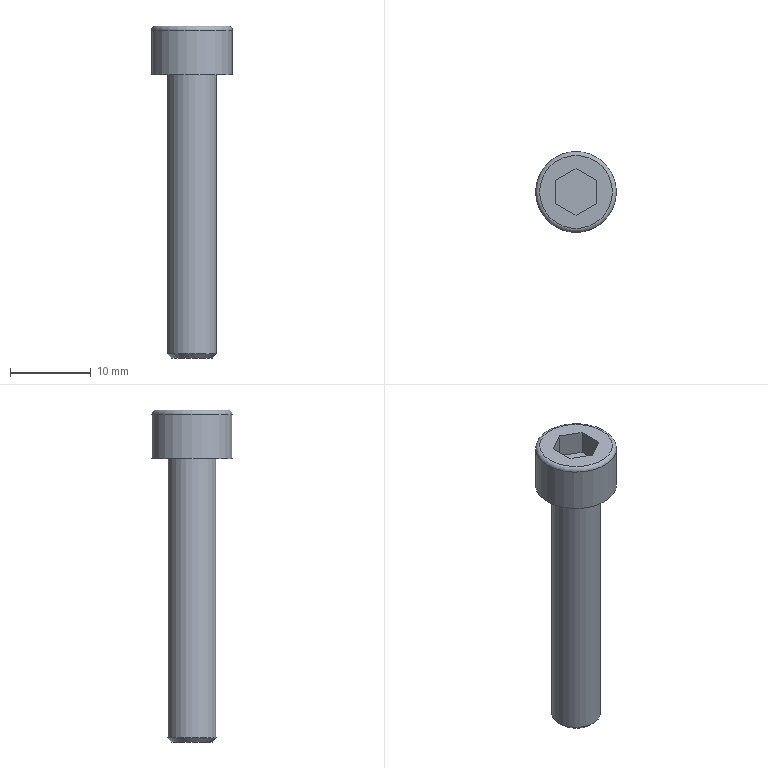Part | STEP file | lll_id66_x_t | 1 solid | 14 faces | box 10 x 10 x 41 mm | volume 1392 mm3 | plane 10 | cylinder 2 | torus 1 | cone 1 | commonest cylinder face diameters 6 x1 10 x1
STEP:
#1=CARTESIAN_POINT('',(24.,58.443,-12.5));
#2=VERTEX_POINT('',#1);
#3=CARTESIAN_POINT('',(21.5,59.887,-12.5));
#4=VERTEX_POINT('',#3);
#5=CARTESIAN_POINT('',(24.,58.443,-12.5));
#6=DIRECTION('',(-0.866,0.5,0.));
#7=VECTOR('',#6,1.);
#8=LINE('',#5,#7);
#9=EDGE_CURVE('',#2,#4,#8,.T.);
#10=ORIENTED_EDGE('',*,*,#9,.F.);
#11=CARTESIAN_POINT('',(24.,55.557,-12.5));
#12=VERTEX_POINT('',#11);
#13=CARTESIAN_POINT('',(24.,55.557,-12.5));
#14=DIRECTION('',(0.,1.,0.));
#15=VECTOR('',#14,1.);
#16=LINE('',#13,#15);
#17=EDGE_CURVE('',#12,#2,#16,.T.);
#18=ORIENTED_EDGE('',*,*,#17,.F.);
#19=CARTESIAN_POINT('',(21.5,54.113,-12.5));
#20=VERTEX_POINT('',#19);
#21=CARTESIAN_POINT('',(21.5,54.113,-12.5));
#22=DIRECTION('',(0.866,0.5,0.));
#23=VECTOR('',#22,1.);
#24=LINE('',#21,#23);
#25=EDGE_CURVE('',#20,#12,#24,.T.);
#26=ORIENTED_EDGE('',*,*,#25,.F.);
#27=CARTESIAN_POINT('',(19.,55.557,-12.5));
#28=VERTEX_POINT('',#27);
#29=CARTESIAN_POINT('',(19.,55.557,-12.5));
#30=DIRECTION('',(0.866,-0.5,0.));
#31=VECTOR('',#30,1.);
#32=LINE('',#29,#31);
#33=EDGE_CURVE('',#28,#20,#32,.T.);
#34=ORIENTED_EDGE('',*,*,#33,.F.);
#35=CARTESIAN_POINT('',(19.,58.443,-12.5));
#36=VERTEX_POINT('',#35);
#37=CARTESIAN_POINT('',(19.,58.443,-12.5));
#38=DIRECTION('',(0.,-1.,0.));
#39=VECTOR('',#38,1.);
#40=LINE('',#37,#39);
#41=EDGE_CURVE('',#36,#28,#40,.T.);
#42=ORIENTED_EDGE('',*,*,#41,.F.);
#43=CARTESIAN_POINT('',(21.5,59.887,-12.5));
#44=DIRECTION('',(-0.866,-0.5,0.));
#45=VECTOR('',#44,1.);
#46=LINE('',#43,#45);
#47=EDGE_CURVE('',#4,#36,#46,.T.);
#48=ORIENTED_EDGE('',*,*,#47,.F.);
#49=EDGE_LOOP('',(#10,#18,#26,#34,#42,#48));
#50=FACE_BOUND('',#49,.T.);
#51=CARTESIAN_POINT('',(26.,57.,-12.5));
#52=VERTEX_POINT('',#51);
#53=CARTESIAN_POINT('',(21.5,57.,-12.5));
#54=DIRECTION('',(0.,0.,1.));
#55=DIRECTION('',(1.,0.,0.));
#56=AXIS2_PLACEMENT_3D('',#53,#54,#55);
#57=CIRCLE('',#56,4.5);
#58=EDGE_CURVE('',#52,#52,#57,.T.);
#59=ORIENTED_EDGE('',*,*,#58,.T.);
#60=EDGE_LOOP('',(#59));
#61=FACE_BOUND('',#60,.T.);
#62=CARTESIAN_POINT('',(21.5,57.,-12.5));
#63=DIRECTION('',(0.,0.,1.));
#64=DIRECTION('',(1.,0.,0.));
#65=AXIS2_PLACEMENT_3D('',#62,#63,#64);
#66=PLANE('',#65);
#67=ADVANCED_FACE('',(#50,#61),#66,.T.);
#68=CARTESIAN_POINT('',(18.5,57.,-18.5));
#69=VERTEX_POINT('',#68);
#70=CARTESIAN_POINT('',(21.5,57.,-18.5));
#71=DIRECTION('',(0.,0.,-1.));
#72=DIRECTION('',(-1.,0.,0.));
#73=AXIS2_PLACEMENT_3D('',#70,#71,#72);
#74=CIRCLE('',#73,3.);
#75=EDGE_CURVE('',#69,#69,#74,.T.);
#76=ORIENTED_EDGE('',*,*,#75,.F.);
#77=EDGE_LOOP('',(#76));
#78=FACE_BOUND('',#77,.T.);
#79=CARTESIAN_POINT('',(26.5,57.,-18.5));
#80=VERTEX_POINT('',#79);
#81=CARTESIAN_POINT('',(21.5,57.,-18.5));
#82=DIRECTION('',(0.,0.,1.));
#83=DIRECTION('',(1.,0.,0.));
#84=AXIS2_PLACEMENT_3D('',#81,#82,#83);
#85=CIRCLE('',#84,5.);
#86=EDGE_CURVE('',#80,#80,#85,.T.);
#87=ORIENTED_EDGE('',*,*,#86,.F.);
#88=EDGE_LOOP('',(#87));
#89=FACE_BOUND('',#88,.T.);
#90=CARTESIAN_POINT('',(21.5,57.,-18.5));
#91=DIRECTION('',(0.,0.,-1.));
#92=DIRECTION('',(-1.,0.,0.));
#93=AXIS2_PLACEMENT_3D('',#90,#91,#92);
#94=PLANE('',#93);
#95=ADVANCED_FACE('',(#78,#89),#94,.T.);
#96=CARTESIAN_POINT('',(26.5,57.,-13.));
#97=VERTEX_POINT('',#96);
#98=CARTESIAN_POINT('',(21.5,57.,-13.));
#99=DIRECTION('',(0.,0.,-1.));
#100=DIRECTION('',(1.,0.,0.));
#101=AXIS2_PLACEMENT_3D('',#98,#99,#100);
#102=CIRCLE('',#101,5.);
#103=EDGE_CURVE('',#97,#97,#102,.T.);
#104=ORIENTED_EDGE('',*,*,#103,.T.);
#105=EDGE_LOOP('',(#104));
#106=FACE_BOUND('',#105,.T.);
#107=ORIENTED_EDGE('',*,*,#86,.T.);
#108=EDGE_LOOP('',(#107));
#109=FACE_BOUND('',#108,.T.);
#110=CARTESIAN_POINT('',(21.5,57.,-18.5));
#111=DIRECTION('',(0.,0.,1.));
#112=DIRECTION('',(1.,0.,0.));
#113=AXIS2_PLACEMENT_3D('',#110,#111,#112);
#114=CYLINDRICAL_SURFACE('',#113,5.);
#115=ADVANCED_FACE('',(#106,#109),#114,.T.);
#116=ORIENTED_EDGE('',*,*,#58,.F.);
#117=EDGE_LOOP('',(#116));
#118=FACE_BOUND('',#117,.T.);
#119=ORIENTED_EDGE('',*,*,#103,.F.);
#120=EDGE_LOOP('',(#119));
#121=FACE_BOUND('',#120,.T.);
#122=CARTESIAN_POINT('',(21.5,57.,-13.));
#123=DIRECTION('',(0.,0.,1.));
#124=DIRECTION('',(1.,0.,0.));
#125=AXIS2_PLACEMENT_3D('',#122,#123,#124);
#126=TOROIDAL_SURFACE('',#125,4.5,0.5);
#127=ADVANCED_FACE('',(#118,#121),#126,.T.);
#128=CARTESIAN_POINT('',(19.,57.,-53.5));
#129=VERTEX_POINT('',#128);
#130=CARTESIAN_POINT('',(21.5,57.,-53.5));
#131=DIRECTION('',(0.,0.,-1.));
#132=DIRECTION('',(-1.,0.,0.));
#133=AXIS2_PLACEMENT_3D('',#130,#131,#132);
#134=CIRCLE('',#133,2.5);
#135=EDGE_CURVE('',#129,#129,#134,.T.);
#136=ORIENTED_EDGE('',*,*,#135,.T.);
#137=EDGE_LOOP('',(#136));
#138=FACE_OUTER_BOUND('',#137,.T.);
#139=CARTESIAN_POINT('',(21.5,57.,-53.5));
#140=DIRECTION('',(0.,0.,-1.));
#141=DIRECTION('',(-1.,0.,0.));
#142=AXIS2_PLACEMENT_3D('',#139,#140,#141);
#143=PLANE('',#142);
#144=ADVANCED_FACE('',(#138),#143,.T.);
#145=ORIENTED_EDGE('',*,*,#75,.T.);
#146=EDGE_LOOP('',(#145));
#147=FACE_BOUND('',#146,.T.);
#148=CARTESIAN_POINT('',(18.5,57.,-53.));
#149=VERTEX_POINT('',#148);
#150=CARTESIAN_POINT('',(21.5,57.,-53.));
#151=DIRECTION('',(0.,0.,1.));
#152=DIRECTION('',(-1.,0.,0.));
#153=AXIS2_PLACEMENT_3D('',#150,#151,#152);
#154=CIRCLE('',#153,3.);
#155=EDGE_CURVE('',#149,#149,#154,.T.);
#156=ORIENTED_EDGE('',*,*,#155,.T.);
#157=EDGE_LOOP('',(#156));
#158=FACE_BOUND('',#157,.T.);
#159=CARTESIAN_POINT('',(21.5,57.,-53.5));
#160=DIRECTION('',(0.,0.,1.));
#161=DIRECTION('',(1.,0.,0.));
#162=AXIS2_PLACEMENT_3D('',#159,#160,#161);
#163=CYLINDRICAL_SURFACE('',#162,3.);
#164=ADVANCED_FACE('',(#147,#158),#163,.T.);
#165=ORIENTED_EDGE('',*,*,#135,.F.);
#166=EDGE_LOOP('',(#165));
#167=FACE_BOUND('',#166,.T.);
#168=ORIENTED_EDGE('',*,*,#155,.F.);
#169=EDGE_LOOP('',(#168));
#170=FACE_BOUND('',#169,.T.);
#171=CARTESIAN_POINT('',(21.5,57.,-53.));
#172=DIRECTION('',(0.,0.,1.));
#173=DIRECTION('',(1.,0.,0.));
#174=AXIS2_PLACEMENT_3D('',#171,#172,#173);
#175=CONICAL_SURFACE('',#174,3.,45.);
#176=ADVANCED_FACE('',(#167,#170),#175,.T.);
#177=CARTESIAN_POINT('',(24.,58.443,-15.5));
#178=VERTEX_POINT('',#177);
#179=CARTESIAN_POINT('',(21.5,59.887,-15.5));
#180=VERTEX_POINT('',#179);
#181=CARTESIAN_POINT('',(24.,58.443,-15.5));
#182=DIRECTION('',(-0.866,0.5,0.));
#183=VECTOR('',#182,1.);
#184=LINE('',#181,#183);
#185=EDGE_CURVE('',#178,#180,#184,.T.);
#186=ORIENTED_EDGE('',*,*,#185,.F.);
#187=CARTESIAN_POINT('',(24.,58.443,-12.5));
#188=DIRECTION('',(0.,0.,-1.));
#189=VECTOR('',#188,1.);
#190=LINE('',#187,#189);
#191=EDGE_CURVE('',#2,#178,#190,.T.);
#192=ORIENTED_EDGE('',*,*,#191,.F.);
#193=ORIENTED_EDGE('',*,*,#9,.T.);
#194=CARTESIAN_POINT('',(21.5,59.887,-12.5));
#195=DIRECTION('',(0.,0.,-1.));
#196=VECTOR('',#195,1.);
#197=LINE('',#194,#196);
#198=EDGE_CURVE('',#4,#180,#197,.T.);
#199=ORIENTED_EDGE('',*,*,#198,.T.);
#200=EDGE_LOOP('',(#186,#192,#193,#199));
#201=FACE_OUTER_BOUND('',#200,.T.);
#202=CARTESIAN_POINT('',(24.,58.443,-12.5));
#203=DIRECTION('',(-0.5,-0.866,0.));
#204=DIRECTION('',(0.866,-0.5,0.));
#205=AXIS2_PLACEMENT_3D('',#202,#203,#204);
#206=PLANE('',#205);
#207=ADVANCED_FACE('',(#201),#206,.T.);
#208=CARTESIAN_POINT('',(19.,58.443,-15.5));
#209=VERTEX_POINT('',#208);
#210=CARTESIAN_POINT('',(21.5,59.887,-15.5));
#211=DIRECTION('',(-0.866,-0.5,0.));
#212=VECTOR('',#211,1.);
#213=LINE('',#210,#212);
#214=EDGE_CURVE('',#180,#209,#213,.T.);
#215=ORIENTED_EDGE('',*,*,#214,.F.);
#216=ORIENTED_EDGE('',*,*,#198,.F.);
#217=ORIENTED_EDGE('',*,*,#47,.T.);
#218=CARTESIAN_POINT('',(19.,58.443,-12.5));
#219=DIRECTION('',(0.,0.,-1.));
#220=VECTOR('',#219,1.);
#221=LINE('',#218,#220);
#222=EDGE_CURVE('',#36,#209,#221,.T.);
#223=ORIENTED_EDGE('',*,*,#222,.T.);
#224=EDGE_LOOP('',(#215,#216,#217,#223));
#225=FACE_OUTER_BOUND('',#224,.T.);
#226=CARTESIAN_POINT('',(21.5,59.887,-12.5));
#227=DIRECTION('',(0.5,-0.866,0.));
#228=DIRECTION('',(0.866,0.5,0.));
#229=AXIS2_PLACEMENT_3D('',#226,#227,#228);
#230=PLANE('',#229);
#231=ADVANCED_FACE('',(#225),#230,.T.);
#232=CARTESIAN_POINT('',(19.,55.557,-15.5));
#233=VERTEX_POINT('',#232);
#234=CARTESIAN_POINT('',(19.,58.443,-15.5));
#235=DIRECTION('',(0.,-1.,0.));
#236=VECTOR('',#235,1.);
#237=LINE('',#234,#236);
#238=EDGE_CURVE('',#209,#233,#237,.T.);
#239=ORIENTED_EDGE('',*,*,#238,.F.);
#240=ORIENTED_EDGE('',*,*,#222,.F.);
#241=ORIENTED_EDGE('',*,*,#41,.T.);
#242=CARTESIAN_POINT('',(19.,55.557,-12.5));
#243=DIRECTION('',(0.,0.,-1.));
#244=VECTOR('',#243,1.);
#245=LINE('',#242,#244);
#246=EDGE_CURVE('',#28,#233,#245,.T.);
#247=ORIENTED_EDGE('',*,*,#246,.T.);
#248=EDGE_LOOP('',(#239,#240,#241,#247));
#249=FACE_OUTER_BOUND('',#248,.T.);
#250=CARTESIAN_POINT('',(19.,58.443,-12.5));
#251=DIRECTION('',(1.,0.,0.));
#252=DIRECTION('',(0.,1.,0.));
#253=AXIS2_PLACEMENT_3D('',#250,#251,#252);
#254=PLANE('',#253);
#255=ADVANCED_FACE('',(#249),#254,.T.);
#256=CARTESIAN_POINT('',(21.5,54.113,-15.5));
#257=VERTEX_POINT('',#256);
#258=CARTESIAN_POINT('',(19.,55.557,-15.5));
#259=DIRECTION('',(0.866,-0.5,0.));
#260=VECTOR('',#259,1.);
#261=LINE('',#258,#260);
#262=EDGE_CURVE('',#233,#257,#261,.T.);
#263=ORIENTED_EDGE('',*,*,#262,.F.);
#264=ORIENTED_EDGE('',*,*,#246,.F.);
#265=ORIENTED_EDGE('',*,*,#33,.T.);
#266=CARTESIAN_POINT('',(21.5,54.113,-12.5));
#267=DIRECTION('',(0.,0.,-1.));
#268=VECTOR('',#267,1.);
#269=LINE('',#266,#268);
#270=EDGE_CURVE('',#20,#257,#269,.T.);
#271=ORIENTED_EDGE('',*,*,#270,.T.);
#272=EDGE_LOOP('',(#263,#264,#265,#271));
#273=FACE_OUTER_BOUND('',#272,.T.);
#274=CARTESIAN_POINT('',(19.,55.557,-12.5));
#275=DIRECTION('',(0.5,0.866,0.));
#276=DIRECTION('',(-0.866,0.5,0.));
#277=AXIS2_PLACEMENT_3D('',#274,#275,#276);
#278=PLANE('',#277);
#279=ADVANCED_FACE('',(#273),#278,.T.);
#280=CARTESIAN_POINT('',(24.,55.557,-15.5));
#281=VERTEX_POINT('',#280);
#282=CARTESIAN_POINT('',(21.5,54.113,-15.5));
#283=DIRECTION('',(0.866,0.5,0.));
#284=VECTOR('',#283,1.);
#285=LINE('',#282,#284);
#286=EDGE_CURVE('',#257,#281,#285,.T.);
#287=ORIENTED_EDGE('',*,*,#286,.F.);
#288=ORIENTED_EDGE('',*,*,#270,.F.);
#289=ORIENTED_EDGE('',*,*,#25,.T.);
#290=CARTESIAN_POINT('',(24.,55.557,-12.5));
#291=DIRECTION('',(0.,0.,-1.));
#292=VECTOR('',#291,1.);
#293=LINE('',#290,#292);
#294=EDGE_CURVE('',#12,#281,#293,.T.);
#295=ORIENTED_EDGE('',*,*,#294,.T.);
#296=EDGE_LOOP('',(#287,#288,#289,#295));
#297=FACE_OUTER_BOUND('',#296,.T.);
#298=CARTESIAN_POINT('',(21.5,54.113,-12.5));
#299=DIRECTION('',(-0.5,0.866,0.));
#300=DIRECTION('',(-0.866,-0.5,0.));
#301=AXIS2_PLACEMENT_3D('',#298,#299,#300);
#302=PLANE('',#301);
#303=ADVANCED_FACE('',(#297),#302,.T.);
#304=CARTESIAN_POINT('',(24.,55.557,-15.5));
#305=DIRECTION('',(0.,1.,0.));
#306=VECTOR('',#305,1.);
#307=LINE('',#304,#306);
#308=EDGE_CURVE('',#281,#178,#307,.T.);
#309=ORIENTED_EDGE('',*,*,#308,.F.);
#310=ORIENTED_EDGE('',*,*,#294,.F.);
#311=ORIENTED_EDGE('',*,*,#17,.T.);
#312=ORIENTED_EDGE('',*,*,#191,.T.);
#313=EDGE_LOOP('',(#309,#310,#311,#312));
#314=FACE_OUTER_BOUND('',#313,.T.);
#315=CARTESIAN_POINT('',(24.,55.557,-12.5));
#316=DIRECTION('',(-1.,0.,0.));
#317=DIRECTION('',(0.,-1.,0.));
#318=AXIS2_PLACEMENT_3D('',#315,#316,#317);
#319=PLANE('',#318);
#320=ADVANCED_FACE('',(#314),#319,.T.);
#321=ORIENTED_EDGE('',*,*,#185,.T.);
#322=ORIENTED_EDGE('',*,*,#214,.T.);
#323=ORIENTED_EDGE('',*,*,#238,.T.);
#324=ORIENTED_EDGE('',*,*,#262,.T.);
#325=ORIENTED_EDGE('',*,*,#286,.T.);
#326=ORIENTED_EDGE('',*,*,#308,.T.);
#327=EDGE_LOOP('',(#321,#322,#323,#324,#325,#326));
#328=FACE_OUTER_BOUND('',#327,.T.);
#329=CARTESIAN_POINT('',(21.5,59.887,-15.5));
#330=DIRECTION('',(0.,0.,1.));
#331=DIRECTION('',(1.,0.,0.));
#332=AXIS2_PLACEMENT_3D('',#329,#330,#331);
#333=PLANE('',#332);
#334=ADVANCED_FACE('',(#328),#333,.T.);
#335=CLOSED_SHELL('',(#67,#95,#115,#127,#144,#164,#176,#207,#231,#255,#279,#303,#320,#334));
#336=MANIFOLD_SOLID_BREP('',#335);
#337=(LENGTH_UNIT()NAMED_UNIT(*)SI_UNIT(.MILLI.,.METRE.));
#338=UNCERTAINTY_MEASURE_WITH_UNIT(LENGTH_MEASURE(0.00002),#337,'','');
#339=(NAMED_UNIT(*)PLANE_ANGLE_UNIT()SI_UNIT($,.RADIAN.));
#340=PLANE_ANGLE_MEASURE_WITH_UNIT(PLANE_ANGLE_MEASURE(0.01745),#339);
#341=DIMENSIONAL_EXPONENTS(0.,0.,0.,0.,0.,0.,0.);
#342=(CONVERSION_BASED_UNIT('DEGREE',#340)NAMED_UNIT(#341)PLANE_ANGLE_UNIT());
#343=(NAMED_UNIT(*)SI_UNIT($,.STERADIAN.)SOLID_ANGLE_UNIT());
#344=(GEOMETRIC_REPRESENTATION_CONTEXT(3)GLOBAL_UNCERTAINTY_ASSIGNED_CONTEXT((#338))GLOBAL_UNIT_ASSIGNED_CONTEXT((#337,#342,#343))REPRESENTATION_CONTEXT('',''));
#345=ADVANCED_BREP_SHAPE_REPRESENTATION('',(#336),#344);